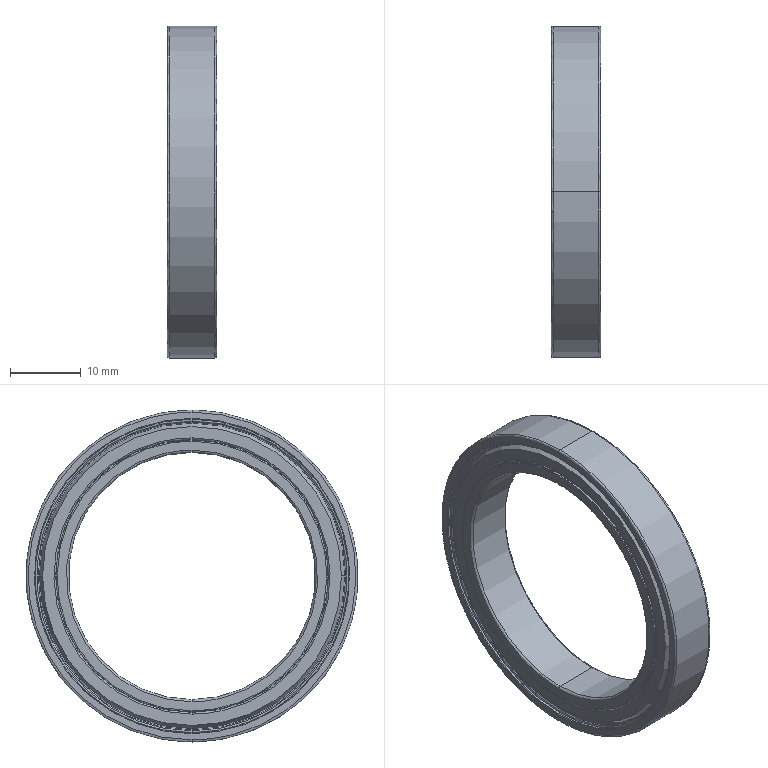Part | SolidWorks | features BaseBody 1 | 1 solid | 136 faces | box 7 x 47 x 47 mm | volume 4480 mm3 | spline 52 | cone 40 | cylinder 32 | plane 12 | commonest cylinder face diameters 37.7 x4 38.4 x4 38.7 x4 39 x4 39.1 x4 43 x4